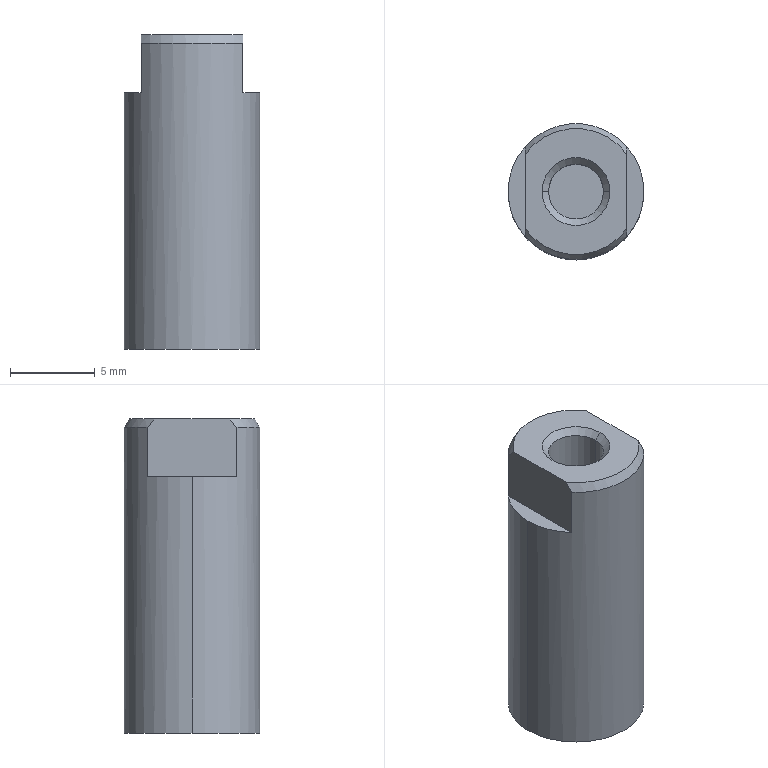Part | STEP file | 11-Rod_A_CDQSB16_10D_A93_0_11 | 1 solid | 15 faces | box 8 x 8 x 18.5 mm | volume 833.39 mm3 | plane 7 | cylinder 4 | cone 4 | commonest cylinder face diameters 3.24 x2 8 x2
STEP:
#1=CARTESIAN_POINT('',(-1.62,0.,-5.));
#2=VERTEX_POINT('',#1);
#3=CARTESIAN_POINT('',(1.62,0.,-5.));
#4=VERTEX_POINT('',#3);
#5=CARTESIAN_POINT('',(0.,0.,-5.));
#6=DIRECTION('',(0.,0.,1.));
#7=DIRECTION('',(1.,0.,0.));
#8=AXIS2_PLACEMENT_3D('',#5,#6,#7);
#9=CIRCLE('',#8,1.62);
#10=EDGE_CURVE('',#2,#4,#9,.T.);
#11=ORIENTED_EDGE('',*,*,#10,.F.);
#12=CARTESIAN_POINT('',(-1.62,0.,3.12));
#13=VERTEX_POINT('',#12);
#14=CARTESIAN_POINT('',(-1.62,0.,-5.));
#15=DIRECTION('',(0.,0.,1.));
#16=VECTOR('',#15,1000.);
#17=LINE('',#14,#16);
#18=EDGE_CURVE('',#2,#13,#17,.T.);
#19=ORIENTED_EDGE('',*,*,#18,.T.);
#20=CARTESIAN_POINT('',(1.62,0.,3.12));
#21=VERTEX_POINT('',#20);
#22=CARTESIAN_POINT('',(0.,0.,3.12));
#23=DIRECTION('',(0.,0.,1.));
#24=DIRECTION('',(1.,0.,0.));
#25=AXIS2_PLACEMENT_3D('',#22,#23,#24);
#26=CIRCLE('',#25,1.62);
#27=EDGE_CURVE('',#13,#21,#26,.T.);
#28=ORIENTED_EDGE('',*,*,#27,.T.);
#29=CARTESIAN_POINT('',(1.62,0.,-5.));
#30=DIRECTION('',(0.,0.,1.));
#31=VECTOR('',#30,1000.);
#32=LINE('',#29,#31);
#33=EDGE_CURVE('',#4,#21,#32,.T.);
#34=ORIENTED_EDGE('',*,*,#33,.F.);
#35=EDGE_LOOP('',(#11,#19,#28,#34));
#36=FACE_OUTER_BOUND('',#35,.T.);
#37=CARTESIAN_POINT('',(0.,0.,-5.));
#38=DIRECTION('',(0.,0.,1.));
#39=DIRECTION('',(1.,0.,0.));
#40=AXIS2_PLACEMENT_3D('',#37,#38,#39);
#41=CYLINDRICAL_SURFACE('',#40,1.62);
#42=ADVANCED_FACE('',(#36),#41,.F.);
#43=ORIENTED_EDGE('',*,*,#27,.F.);
#44=CARTESIAN_POINT('',(-2.,0.,3.5));
#45=VERTEX_POINT('',#44);
#46=CARTESIAN_POINT('',(-1.62,0.,3.12));
#47=DIRECTION('',(-0.7071,0.,0.7071));
#48=VECTOR('',#47,1000.);
#49=LINE('',#46,#48);
#50=EDGE_CURVE('',#13,#45,#49,.T.);
#51=ORIENTED_EDGE('',*,*,#50,.T.);
#52=CARTESIAN_POINT('',(2.,0.,3.5));
#53=VERTEX_POINT('',#52);
#54=CARTESIAN_POINT('',(0.,0.,3.5));
#55=DIRECTION('',(0.,0.,1.));
#56=DIRECTION('',(-1.,0.,0.));
#57=AXIS2_PLACEMENT_3D('',#54,#55,#56);
#58=CIRCLE('',#57,2.);
#59=EDGE_CURVE('',#45,#53,#58,.T.);
#60=ORIENTED_EDGE('',*,*,#59,.T.);
#61=CARTESIAN_POINT('',(1.62,0.,3.12));
#62=DIRECTION('',(0.7071,0.,0.7071));
#63=VECTOR('',#62,1000.);
#64=LINE('',#61,#63);
#65=EDGE_CURVE('',#21,#53,#64,.T.);
#66=ORIENTED_EDGE('',*,*,#65,.F.);
#67=EDGE_LOOP('',(#43,#51,#60,#66));
#68=FACE_OUTER_BOUND('',#67,.T.);
#69=CARTESIAN_POINT('',(0.,0.,3.12));
#70=DIRECTION('',(0.,0.,1.));
#71=DIRECTION('',(1.,0.,0.));
#72=AXIS2_PLACEMENT_3D('',#69,#70,#71);
#73=CONICAL_SURFACE('',#72,1.62,0.7854);
#74=ADVANCED_FACE('',(#68),#73,.F.);
#75=CARTESIAN_POINT('',(4.,0.,-15.));
#76=VERTEX_POINT('',#75);
#77=CARTESIAN_POINT('',(-4.,0.,-15.));
#78=VERTEX_POINT('',#77);
#79=CARTESIAN_POINT('',(0.,0.,-15.));
#80=DIRECTION('',(0.,0.,1.));
#81=DIRECTION('',(1.,0.,0.));
#82=AXIS2_PLACEMENT_3D('',#79,#80,#81);
#83=CIRCLE('',#82,4.);
#84=EDGE_CURVE('',#76,#78,#83,.T.);
#85=ORIENTED_EDGE('',*,*,#84,.T.);
#86=CARTESIAN_POINT('',(-4.,0.,0.1));
#87=VERTEX_POINT('',#86);
#88=CARTESIAN_POINT('',(-4.,0.,-15.));
#89=DIRECTION('',(0.,0.,1.));
#90=VECTOR('',#89,1000.);
#91=LINE('',#88,#90);
#92=EDGE_CURVE('',#78,#87,#91,.T.);
#93=ORIENTED_EDGE('',*,*,#92,.T.);
#94=CARTESIAN_POINT('',(-3.,2.646,0.1));
#95=VERTEX_POINT('',#94);
#96=CARTESIAN_POINT('',(0.,0.,0.1));
#97=DIRECTION('',(0.,0.,1.));
#98=DIRECTION('',(1.,0.,0.));
#99=AXIS2_PLACEMENT_3D('',#96,#97,#98);
#100=CIRCLE('',#99,4.);
#101=EDGE_CURVE('',#95,#87,#100,.T.);
#102=ORIENTED_EDGE('',*,*,#101,.F.);
#103=CARTESIAN_POINT('',(-3.,2.646,3.));
#104=VERTEX_POINT('',#103);
#105=CARTESIAN_POINT('',(-3.,2.646,-15.));
#106=DIRECTION('',(0.,0.,1.));
#107=VECTOR('',#106,1000.);
#108=LINE('',#105,#107);
#109=EDGE_CURVE('',#95,#104,#108,.T.);
#110=ORIENTED_EDGE('',*,*,#109,.T.);
#111=CARTESIAN_POINT('',(3.,2.646,3.));
#112=VERTEX_POINT('',#111);
#113=CARTESIAN_POINT('',(0.,0.,3.));
#114=DIRECTION('',(0.,0.,1.));
#115=DIRECTION('',(1.,0.,0.));
#116=AXIS2_PLACEMENT_3D('',#113,#114,#115);
#117=CIRCLE('',#116,4.);
#118=EDGE_CURVE('',#112,#104,#117,.T.);
#119=ORIENTED_EDGE('',*,*,#118,.F.);
#120=CARTESIAN_POINT('',(3.,2.646,0.1));
#121=VERTEX_POINT('',#120);
#122=CARTESIAN_POINT('',(3.,2.646,-15.));
#123=DIRECTION('',(0.,0.,-1.));
#124=VECTOR('',#123,1000.);
#125=LINE('',#122,#124);
#126=EDGE_CURVE('',#112,#121,#125,.T.);
#127=ORIENTED_EDGE('',*,*,#126,.T.);
#128=CARTESIAN_POINT('',(4.,0.,0.1));
#129=VERTEX_POINT('',#128);
#130=CARTESIAN_POINT('',(0.,0.,0.1));
#131=DIRECTION('',(0.,0.,1.));
#132=DIRECTION('',(1.,0.,0.));
#133=AXIS2_PLACEMENT_3D('',#130,#131,#132);
#134=CIRCLE('',#133,4.);
#135=EDGE_CURVE('',#129,#121,#134,.T.);
#136=ORIENTED_EDGE('',*,*,#135,.F.);
#137=CARTESIAN_POINT('',(4.,0.,-15.));
#138=DIRECTION('',(0.,0.,1.));
#139=VECTOR('',#138,1000.);
#140=LINE('',#137,#139);
#141=EDGE_CURVE('',#76,#129,#140,.T.);
#142=ORIENTED_EDGE('',*,*,#141,.F.);
#143=EDGE_LOOP('',(#85,#93,#102,#110,#119,#127,#136,#142));
#144=FACE_OUTER_BOUND('',#143,.T.);
#145=CARTESIAN_POINT('',(0.,0.,-15.));
#146=DIRECTION('',(0.,0.,1.));
#147=DIRECTION('',(1.,0.,0.));
#148=AXIS2_PLACEMENT_3D('',#145,#146,#147);
#149=CYLINDRICAL_SURFACE('',#148,4.);
#150=ADVANCED_FACE('',(#144),#149,.T.);
#151=CARTESIAN_POINT('',(-3.,-2.646,3.));
#152=VERTEX_POINT('',#151);
#153=CARTESIAN_POINT('',(3.,-2.646,3.));
#154=VERTEX_POINT('',#153);
#155=CARTESIAN_POINT('',(0.,0.,3.));
#156=DIRECTION('',(0.,0.,1.));
#157=DIRECTION('',(1.,0.,0.));
#158=AXIS2_PLACEMENT_3D('',#155,#156,#157);
#159=CIRCLE('',#158,4.);
#160=EDGE_CURVE('',#152,#154,#159,.T.);
#161=ORIENTED_EDGE('',*,*,#160,.T.);
#162=CARTESIAN_POINT('',(3.,-2.185,3.5));
#163=VERTEX_POINT('',#162);
#164=CARTESIAN_POINT('',(3.,-2.646,3.));
#165=CARTESIAN_POINT('',(3.,-2.497,3.171));
#166=CARTESIAN_POINT('',(3.,-2.344,3.338));
#167=CARTESIAN_POINT('',(3.,-2.185,3.5));
#168=B_SPLINE_CURVE_WITH_KNOTS('',3,(#164,#165,#166,#167),.UNSPECIFIED.,.F.,.F.,(4,4),(0.005913,0.006593),.UNSPECIFIED.);
#169=EDGE_CURVE('',#154,#163,#168,.T.);
#170=ORIENTED_EDGE('',*,*,#169,.T.);
#171=CARTESIAN_POINT('',(-3.,-2.185,3.5));
#172=VERTEX_POINT('',#171);
#173=CARTESIAN_POINT('',(0.,0.,3.5));
#174=DIRECTION('',(0.,0.,1.));
#175=DIRECTION('',(1.,0.,0.));
#176=AXIS2_PLACEMENT_3D('',#173,#174,#175);
#177=CIRCLE('',#176,3.711);
#178=EDGE_CURVE('',#172,#163,#177,.T.);
#179=ORIENTED_EDGE('',*,*,#178,.F.);
#180=CARTESIAN_POINT('',(-3.,-2.185,3.5));
#181=CARTESIAN_POINT('',(-3.,-2.344,3.338));
#182=CARTESIAN_POINT('',(-3.,-2.497,3.171));
#183=CARTESIAN_POINT('',(-3.,-2.646,3.));
#184=B_SPLINE_CURVE_WITH_KNOTS('',3,(#180,#181,#182,#183),.UNSPECIFIED.,.F.,.F.,(4,4),(0.01174,0.01243),.UNSPECIFIED.);
#185=EDGE_CURVE('',#172,#152,#184,.T.);
#186=ORIENTED_EDGE('',*,*,#185,.T.);
#187=EDGE_LOOP('',(#161,#170,#179,#186));
#188=FACE_OUTER_BOUND('',#187,.T.);
#189=CARTESIAN_POINT('',(0.,0.,3.));
#190=DIRECTION('',(0.,0.,-1.));
#191=DIRECTION('',(-1.,0.,0.));
#192=AXIS2_PLACEMENT_3D('',#189,#190,#191);
#193=CONICAL_SURFACE('',#192,4.,0.5236);
#194=ADVANCED_FACE('',(#188),#193,.T.);
#195=ORIENTED_EDGE('',*,*,#178,.T.);
#196=CARTESIAN_POINT('',(3.,2.185,3.5));
#197=VERTEX_POINT('',#196);
#198=CARTESIAN_POINT('',(3.,6.,3.5));
#199=DIRECTION('',(0.,-1.,0.));
#200=VECTOR('',#199,1000.);
#201=LINE('',#198,#200);
#202=EDGE_CURVE('',#197,#163,#201,.T.);
#203=ORIENTED_EDGE('',*,*,#202,.F.);
#204=CARTESIAN_POINT('',(-3.,2.185,3.5));
#205=VERTEX_POINT('',#204);
#206=CARTESIAN_POINT('',(0.,0.,3.5));
#207=DIRECTION('',(0.,0.,1.));
#208=DIRECTION('',(1.,0.,0.));
#209=AXIS2_PLACEMENT_3D('',#206,#207,#208);
#210=CIRCLE('',#209,3.711);
#211=EDGE_CURVE('',#197,#205,#210,.T.);
#212=ORIENTED_EDGE('',*,*,#211,.T.);
#213=CARTESIAN_POINT('',(-3.,-5.,3.5));
#214=DIRECTION('',(0.,1.,0.));
#215=VECTOR('',#214,1000.);
#216=LINE('',#213,#215);
#217=EDGE_CURVE('',#172,#205,#216,.T.);
#218=ORIENTED_EDGE('',*,*,#217,.F.);
#219=EDGE_LOOP('',(#195,#203,#212,#218));
#220=FACE_OUTER_BOUND('',#219,.T.);
#221=CARTESIAN_POINT('',(0.,0.,3.5));
#222=DIRECTION('',(0.,0.,1.));
#223=DIRECTION('',(-1.,0.,0.));
#224=AXIS2_PLACEMENT_3D('',#221,#222,#223);
#225=CIRCLE('',#224,2.);
#226=EDGE_CURVE('',#53,#45,#225,.T.);
#227=ORIENTED_EDGE('',*,*,#226,.F.);
#228=ORIENTED_EDGE('',*,*,#59,.F.);
#229=EDGE_LOOP('',(#227,#228));
#230=FACE_BOUND('',#229,.T.);
#231=CARTESIAN_POINT('',(0.,0.,3.5));
#232=DIRECTION('',(0.,0.,-1.));
#233=DIRECTION('',(-1.,0.,0.));
#234=AXIS2_PLACEMENT_3D('',#231,#232,#233);
#235=PLANE('',#234);
#236=ADVANCED_FACE('',(#220,#230),#235,.F.);
#237=ORIENTED_EDGE('',*,*,#211,.F.);
#238=CARTESIAN_POINT('',(3.,2.185,3.5));
#239=CARTESIAN_POINT('',(3.,2.344,3.338));
#240=CARTESIAN_POINT('',(3.,2.497,3.171));
#241=CARTESIAN_POINT('',(3.,2.646,3.));
#242=B_SPLINE_CURVE_WITH_KNOTS('',3,(#238,#239,#240,#241),.UNSPECIFIED.,.F.,.F.,(4,4),(0.01174,0.01243),.UNSPECIFIED.);
#243=EDGE_CURVE('',#197,#112,#242,.T.);
#244=ORIENTED_EDGE('',*,*,#243,.T.);
#245=ORIENTED_EDGE('',*,*,#118,.T.);
#246=CARTESIAN_POINT('',(-3.,2.646,3.));
#247=CARTESIAN_POINT('',(-3.,2.497,3.171));
#248=CARTESIAN_POINT('',(-3.,2.344,3.338));
#249=CARTESIAN_POINT('',(-3.,2.185,3.5));
#250=B_SPLINE_CURVE_WITH_KNOTS('',3,(#246,#247,#248,#249),.UNSPECIFIED.,.F.,.F.,(4,4),(0.005913,0.006593),.UNSPECIFIED.);
#251=EDGE_CURVE('',#104,#205,#250,.T.);
#252=ORIENTED_EDGE('',*,*,#251,.T.);
#253=EDGE_LOOP('',(#237,#244,#245,#252));
#254=FACE_OUTER_BOUND('',#253,.T.);
#255=CARTESIAN_POINT('',(0.,0.,3.));
#256=DIRECTION('',(0.,0.,-1.));
#257=DIRECTION('',(-1.,0.,0.));
#258=AXIS2_PLACEMENT_3D('',#255,#256,#257);
#259=CONICAL_SURFACE('',#258,4.,0.5236);
#260=ADVANCED_FACE('',(#254),#259,.T.);
#261=ORIENTED_EDGE('',*,*,#92,.F.);
#262=CARTESIAN_POINT('',(0.,0.,-15.));
#263=DIRECTION('',(0.,0.,1.));
#264=DIRECTION('',(1.,0.,0.));
#265=AXIS2_PLACEMENT_3D('',#262,#263,#264);
#266=CIRCLE('',#265,4.);
#267=EDGE_CURVE('',#78,#76,#266,.T.);
#268=ORIENTED_EDGE('',*,*,#267,.T.);
#269=ORIENTED_EDGE('',*,*,#141,.T.);
#270=CARTESIAN_POINT('',(3.,-2.646,0.1));
#271=VERTEX_POINT('',#270);
#272=CARTESIAN_POINT('',(0.,0.,0.1));
#273=DIRECTION('',(0.,0.,1.));
#274=DIRECTION('',(1.,0.,0.));
#275=AXIS2_PLACEMENT_3D('',#272,#273,#274);
#276=CIRCLE('',#275,4.);
#277=EDGE_CURVE('',#271,#129,#276,.T.);
#278=ORIENTED_EDGE('',*,*,#277,.F.);
#279=CARTESIAN_POINT('',(3.,-2.646,-15.));
#280=DIRECTION('',(0.,0.,1.));
#281=VECTOR('',#280,1000.);
#282=LINE('',#279,#281);
#283=EDGE_CURVE('',#271,#154,#282,.T.);
#284=ORIENTED_EDGE('',*,*,#283,.T.);
#285=ORIENTED_EDGE('',*,*,#160,.F.);
#286=CARTESIAN_POINT('',(-3.,-2.646,0.1));
#287=VERTEX_POINT('',#286);
#288=CARTESIAN_POINT('',(-3.,-2.646,-15.));
#289=DIRECTION('',(0.,0.,-1.));
#290=VECTOR('',#289,1000.);
#291=LINE('',#288,#290);
#292=EDGE_CURVE('',#152,#287,#291,.T.);
#293=ORIENTED_EDGE('',*,*,#292,.T.);
#294=CARTESIAN_POINT('',(0.,0.,0.1));
#295=DIRECTION('',(0.,0.,1.));
#296=DIRECTION('',(1.,0.,0.));
#297=AXIS2_PLACEMENT_3D('',#294,#295,#296);
#298=CIRCLE('',#297,4.);
#299=EDGE_CURVE('',#87,#287,#298,.T.);
#300=ORIENTED_EDGE('',*,*,#299,.F.);
#301=EDGE_LOOP('',(#261,#268,#269,#278,#284,#285,#293,#300));
#302=FACE_OUTER_BOUND('',#301,.T.);
#303=CARTESIAN_POINT('',(0.,0.,-15.));
#304=DIRECTION('',(0.,0.,1.));
#305=DIRECTION('',(1.,0.,0.));
#306=AXIS2_PLACEMENT_3D('',#303,#304,#305);
#307=CYLINDRICAL_SURFACE('',#306,4.);
#308=ADVANCED_FACE('',(#302),#307,.T.);
#309=ORIENTED_EDGE('',*,*,#84,.F.);
#310=ORIENTED_EDGE('',*,*,#267,.F.);
#311=EDGE_LOOP('',(#309,#310));
#312=FACE_OUTER_BOUND('',#311,.T.);
#313=CARTESIAN_POINT('',(0.,4.,-15.));
#314=DIRECTION('',(0.,0.,1.));
#315=DIRECTION('',(1.,0.,0.));
#316=AXIS2_PLACEMENT_3D('',#313,#314,#315);
#317=PLANE('',#316);
#318=ADVANCED_FACE('',(#312),#317,.F.);
#319=ORIENTED_EDGE('',*,*,#50,.F.);
#320=CARTESIAN_POINT('',(0.,0.,3.12));
#321=DIRECTION('',(0.,0.,1.));
#322=DIRECTION('',(1.,0.,0.));
#323=AXIS2_PLACEMENT_3D('',#320,#321,#322);
#324=CIRCLE('',#323,1.62);
#325=EDGE_CURVE('',#21,#13,#324,.T.);
#326=ORIENTED_EDGE('',*,*,#325,.F.);
#327=ORIENTED_EDGE('',*,*,#65,.T.);
#328=ORIENTED_EDGE('',*,*,#226,.T.);
#329=EDGE_LOOP('',(#319,#326,#327,#328));
#330=FACE_OUTER_BOUND('',#329,.T.);
#331=CARTESIAN_POINT('',(0.,0.,3.12));
#332=DIRECTION('',(0.,0.,1.));
#333=DIRECTION('',(1.,0.,0.));
#334=AXIS2_PLACEMENT_3D('',#331,#332,#333);
#335=CONICAL_SURFACE('',#334,1.62,0.7854);
#336=ADVANCED_FACE('',(#330),#335,.F.);
#337=ORIENTED_EDGE('',*,*,#18,.F.);
#338=CARTESIAN_POINT('',(0.,0.,-5.));
#339=DIRECTION('',(0.,0.,1.));
#340=DIRECTION('',(1.,0.,0.));
#341=AXIS2_PLACEMENT_3D('',#338,#339,#340);
#342=CIRCLE('',#341,1.62);
#343=EDGE_CURVE('',#4,#2,#342,.T.);
#344=ORIENTED_EDGE('',*,*,#343,.F.);
#345=ORIENTED_EDGE('',*,*,#33,.T.);
#346=ORIENTED_EDGE('',*,*,#325,.T.);
#347=EDGE_LOOP('',(#337,#344,#345,#346));
#348=FACE_OUTER_BOUND('',#347,.T.);
#349=CARTESIAN_POINT('',(0.,0.,-5.));
#350=DIRECTION('',(0.,0.,1.));
#351=DIRECTION('',(1.,0.,0.));
#352=AXIS2_PLACEMENT_3D('',#349,#350,#351);
#353=CYLINDRICAL_SURFACE('',#352,1.62);
#354=ADVANCED_FACE('',(#348),#353,.F.);
#355=ORIENTED_EDGE('',*,*,#343,.T.);
#356=ORIENTED_EDGE('',*,*,#10,.T.);
#357=EDGE_LOOP('',(#355,#356));
#358=FACE_OUTER_BOUND('',#357,.T.);
#359=CARTESIAN_POINT('',(0.,1.62,-5.));
#360=DIRECTION('',(0.,0.,1.));
#361=DIRECTION('',(1.,0.,0.));
#362=AXIS2_PLACEMENT_3D('',#359,#360,#361);
#363=PLANE('',#362);
#364=ADVANCED_FACE('',(#358),#363,.T.);
#365=ORIENTED_EDGE('',*,*,#277,.T.);
#366=ORIENTED_EDGE('',*,*,#135,.T.);
#367=CARTESIAN_POINT('',(3.,6.,0.1));
#368=DIRECTION('',(0.,-1.,0.));
#369=VECTOR('',#368,1000.);
#370=LINE('',#367,#369);
#371=EDGE_CURVE('',#121,#271,#370,.T.);
#372=ORIENTED_EDGE('',*,*,#371,.T.);
#373=EDGE_LOOP('',(#365,#366,#372));
#374=FACE_OUTER_BOUND('',#373,.T.);
#375=CARTESIAN_POINT('',(-8.,8.,0.1));
#376=DIRECTION('',(0.,0.,1.));
#377=DIRECTION('',(1.,0.,0.));
#378=AXIS2_PLACEMENT_3D('',#375,#376,#377);
#379=PLANE('',#378);
#380=ADVANCED_FACE('',(#374),#379,.T.);
#381=ORIENTED_EDGE('',*,*,#283,.F.);
#382=ORIENTED_EDGE('',*,*,#371,.F.);
#383=ORIENTED_EDGE('',*,*,#126,.F.);
#384=ORIENTED_EDGE('',*,*,#243,.F.);
#385=ORIENTED_EDGE('',*,*,#202,.T.);
#386=ORIENTED_EDGE('',*,*,#169,.F.);
#387=EDGE_LOOP('',(#381,#382,#383,#384,#385,#386));
#388=FACE_OUTER_BOUND('',#387,.T.);
#389=CARTESIAN_POINT('',(3.,6.,0.1));
#390=DIRECTION('',(-1.,0.,0.));
#391=DIRECTION('',(0.,0.,1.));
#392=AXIS2_PLACEMENT_3D('',#389,#390,#391);
#393=PLANE('',#392);
#394=ADVANCED_FACE('',(#388),#393,.F.);
#395=ORIENTED_EDGE('',*,*,#109,.F.);
#396=CARTESIAN_POINT('',(-3.,-5.,0.1));
#397=DIRECTION('',(0.,1.,0.));
#398=VECTOR('',#397,1000.);
#399=LINE('',#396,#398);
#400=EDGE_CURVE('',#287,#95,#399,.T.);
#401=ORIENTED_EDGE('',*,*,#400,.F.);
#402=ORIENTED_EDGE('',*,*,#292,.F.);
#403=ORIENTED_EDGE('',*,*,#185,.F.);
#404=ORIENTED_EDGE('',*,*,#217,.T.);
#405=ORIENTED_EDGE('',*,*,#251,.F.);
#406=EDGE_LOOP('',(#395,#401,#402,#403,#404,#405));
#407=FACE_OUTER_BOUND('',#406,.T.);
#408=CARTESIAN_POINT('',(-3.,-5.,0.1));
#409=DIRECTION('',(1.,0.,0.));
#410=DIRECTION('',(0.,0.,-1.));
#411=AXIS2_PLACEMENT_3D('',#408,#409,#410);
#412=PLANE('',#411);
#413=ADVANCED_FACE('',(#407),#412,.F.);
#414=ORIENTED_EDGE('',*,*,#101,.T.);
#415=ORIENTED_EDGE('',*,*,#299,.T.);
#416=ORIENTED_EDGE('',*,*,#400,.T.);
#417=EDGE_LOOP('',(#414,#415,#416));
#418=FACE_OUTER_BOUND('',#417,.T.);
#419=CARTESIAN_POINT('',(-8.,8.,0.1));
#420=DIRECTION('',(0.,0.,1.));
#421=DIRECTION('',(1.,0.,0.));
#422=AXIS2_PLACEMENT_3D('',#419,#420,#421);
#423=PLANE('',#422);
#424=ADVANCED_FACE('',(#418),#423,.T.);
#425=CLOSED_SHELL('',(#42,#74,#150,#194,#236,#260,#308,#318,#336,#354,#364,#380,#394,#413,#424));
#426=MANIFOLD_SOLID_BREP('',#425);
#427=CARTESIAN_POINT('',(0.,0.,0.));
#428=DIRECTION('',(0.,0.,1.));
#429=DIRECTION('',(1.,0.,0.));
#430=AXIS2_PLACEMENT_3D('',#427,#428,#429);
#431=(LENGTH_UNIT()NAMED_UNIT(*)SI_UNIT(.MILLI.,.METRE.));
#432=UNCERTAINTY_MEASURE_WITH_UNIT(LENGTH_MEASURE(0.00001),#431,'','');
#433=(NAMED_UNIT(*)PLANE_ANGLE_UNIT()SI_UNIT($,.RADIAN.));
#434=(NAMED_UNIT(*)SI_UNIT($,.STERADIAN.)SOLID_ANGLE_UNIT());
#435=(GEOMETRIC_REPRESENTATION_CONTEXT(3)GLOBAL_UNCERTAINTY_ASSIGNED_CONTEXT((#432))GLOBAL_UNIT_ASSIGNED_CONTEXT((#431,#433,#434))REPRESENTATION_CONTEXT('',''));
#436=ADVANCED_BREP_SHAPE_REPRESENTATION('',(#426,#430),#435);